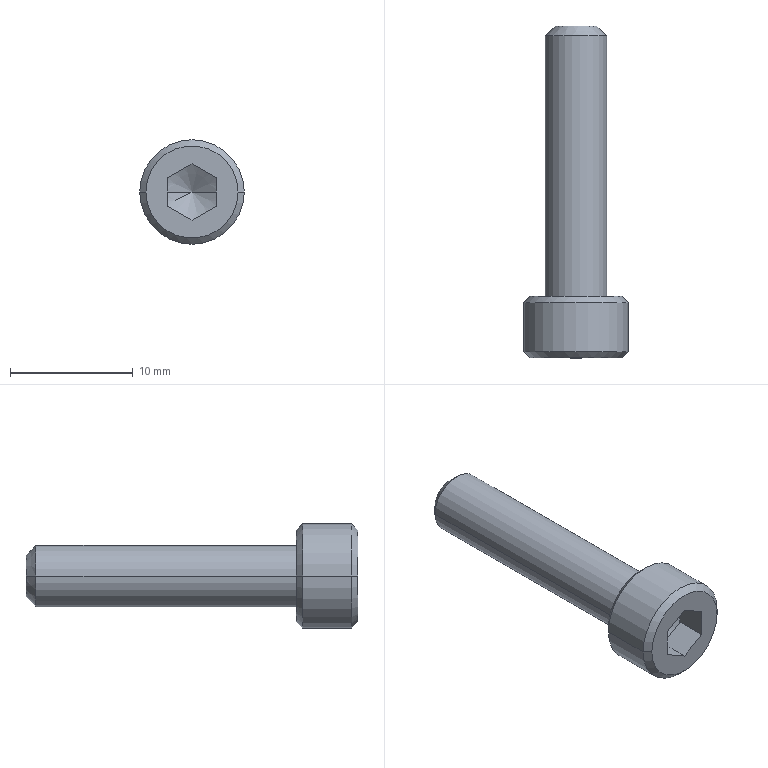Part | STEP file | BB62-M5-22L-44 | 1 solid | 27 faces | box 8.5 x 27 x 8.5 mm | volume 663.468 mm3 | plane 15 | cone 8 | cylinder 4 | commonest cylinder face diameters 5 x2 8.5 x2
STEP:
#1=CARTESIAN_POINT('',(0.,-1.178,0.));
#2=VERTEX_POINT('',#1);
#3=CARTESIAN_POINT('',(2.29,-2.5,0.));
#4=VERTEX_POINT('',#3);
#5=CARTESIAN_POINT('',(0.,-1.178,0.));
#6=DIRECTION('',(0.866,-0.5,0.));
#7=VECTOR('',#6,1000.);
#8=LINE('',#5,#7);
#9=EDGE_CURVE('',#2,#4,#8,.T.);
#10=ORIENTED_EDGE('',*,*,#9,.F.);
#11=CARTESIAN_POINT('',(-2.29,-2.5,0.));
#12=VERTEX_POINT('',#11);
#13=CARTESIAN_POINT('',(0.,-1.178,0.));
#14=DIRECTION('',(-0.866,-0.5,0.));
#15=VECTOR('',#14,1000.);
#16=LINE('',#13,#15);
#17=EDGE_CURVE('',#2,#12,#16,.T.);
#18=ORIENTED_EDGE('',*,*,#17,.T.);
#19=CARTESIAN_POINT('',(-1.983,-2.5,-1.145));
#20=VERTEX_POINT('',#19);
#21=CARTESIAN_POINT('',(0.,-2.5,0.));
#22=DIRECTION('',(0.,-1.,0.));
#23=DIRECTION('',(-1.,0.,0.));
#24=AXIS2_PLACEMENT_3D('',#21,#22,#23);
#25=CIRCLE('',#24,2.29);
#26=EDGE_CURVE('',#12,#20,#25,.T.);
#27=ORIENTED_EDGE('',*,*,#26,.T.);
#28=CARTESIAN_POINT('',(0.,-2.5,-2.29));
#29=VERTEX_POINT('',#28);
#30=CARTESIAN_POINT('',(0.,-2.5,0.));
#31=DIRECTION('',(0.,-1.,0.));
#32=DIRECTION('',(-1.,0.,0.));
#33=AXIS2_PLACEMENT_3D('',#30,#31,#32);
#34=CIRCLE('',#33,2.29);
#35=EDGE_CURVE('',#20,#29,#34,.T.);
#36=ORIENTED_EDGE('',*,*,#35,.T.);
#37=CARTESIAN_POINT('',(1.983,-2.5,-1.145));
#38=VERTEX_POINT('',#37);
#39=CARTESIAN_POINT('',(0.,-2.5,0.));
#40=DIRECTION('',(0.,-1.,0.));
#41=DIRECTION('',(-1.,0.,0.));
#42=AXIS2_PLACEMENT_3D('',#39,#40,#41);
#43=CIRCLE('',#42,2.29);
#44=EDGE_CURVE('',#29,#38,#43,.T.);
#45=ORIENTED_EDGE('',*,*,#44,.T.);
#46=CARTESIAN_POINT('',(0.,-2.5,0.));
#47=DIRECTION('',(0.,-1.,0.));
#48=DIRECTION('',(-1.,0.,0.));
#49=AXIS2_PLACEMENT_3D('',#46,#47,#48);
#50=CIRCLE('',#49,2.29);
#51=EDGE_CURVE('',#38,#4,#50,.T.);
#52=ORIENTED_EDGE('',*,*,#51,.T.);
#53=EDGE_LOOP('',(#10,#18,#27,#36,#45,#52));
#54=FACE_OUTER_BOUND('',#53,.T.);
#55=CARTESIAN_POINT('',(0.,-1001.178,0.));
#56=DIRECTION('',(0.,-1.,0.));
#57=DIRECTION('',(1.,0.,0.));
#58=AXIS2_PLACEMENT_3D('',#55,#56,#57);
#59=CONICAL_SURFACE('',#58,1732.051,1.047);
#60=ADVANCED_FACE('',(#54),#59,.F.);
#61=CARTESIAN_POINT('',(-1.7,22.,0.));
#62=VERTEX_POINT('',#61);
#63=CARTESIAN_POINT('',(1.7,22.,0.));
#64=VERTEX_POINT('',#63);
#65=CARTESIAN_POINT('',(0.,22.,0.));
#66=DIRECTION('',(0.,1.,0.));
#67=DIRECTION('',(1.,0.,0.));
#68=AXIS2_PLACEMENT_3D('',#65,#66,#67);
#69=CIRCLE('',#68,1.7);
#70=EDGE_CURVE('',#62,#64,#69,.T.);
#71=ORIENTED_EDGE('',*,*,#70,.F.);
#72=CARTESIAN_POINT('',(-2.5,21.2,0.));
#73=VERTEX_POINT('',#72);
#74=CARTESIAN_POINT('',(-1.7,22.,0.));
#75=DIRECTION('',(-0.7071,-0.7071,0.));
#76=VECTOR('',#75,1000.);
#77=LINE('',#74,#76);
#78=EDGE_CURVE('',#62,#73,#77,.T.);
#79=ORIENTED_EDGE('',*,*,#78,.T.);
#80=CARTESIAN_POINT('',(2.5,21.2,0.));
#81=VERTEX_POINT('',#80);
#82=CARTESIAN_POINT('',(0.,21.2,0.));
#83=DIRECTION('',(0.,-1.,0.));
#84=DIRECTION('',(-1.,0.,0.));
#85=AXIS2_PLACEMENT_3D('',#82,#83,#84);
#86=CIRCLE('',#85,2.5);
#87=EDGE_CURVE('',#81,#73,#86,.T.);
#88=ORIENTED_EDGE('',*,*,#87,.F.);
#89=CARTESIAN_POINT('',(1.7,22.,0.));
#90=DIRECTION('',(0.7071,-0.7071,0.));
#91=VECTOR('',#90,1000.);
#92=LINE('',#89,#91);
#93=EDGE_CURVE('',#64,#81,#92,.T.);
#94=ORIENTED_EDGE('',*,*,#93,.F.);
#95=EDGE_LOOP('',(#71,#79,#88,#94));
#96=FACE_OUTER_BOUND('',#95,.T.);
#97=CARTESIAN_POINT('',(0.,22.,0.));
#98=DIRECTION('',(0.,-1.,0.));
#99=DIRECTION('',(1.,0.,0.));
#100=AXIS2_PLACEMENT_3D('',#97,#98,#99);
#101=CONICAL_SURFACE('',#100,1.7,0.7854);
#102=ADVANCED_FACE('',(#96),#101,.T.);
#103=ORIENTED_EDGE('',*,*,#87,.T.);
#104=CARTESIAN_POINT('',(-2.5,0.,0.));
#105=VERTEX_POINT('',#104);
#106=CARTESIAN_POINT('',(-2.5,21.2,0.));
#107=DIRECTION('',(0.,-1.,0.));
#108=VECTOR('',#107,1000.);
#109=LINE('',#106,#108);
#110=EDGE_CURVE('',#73,#105,#109,.T.);
#111=ORIENTED_EDGE('',*,*,#110,.T.);
#112=CARTESIAN_POINT('',(2.5,0.,0.));
#113=VERTEX_POINT('',#112);
#114=CARTESIAN_POINT('',(0.,0.,0.));
#115=DIRECTION('',(0.,-1.,0.));
#116=DIRECTION('',(-1.,0.,0.));
#117=AXIS2_PLACEMENT_3D('',#114,#115,#116);
#118=CIRCLE('',#117,2.5);
#119=EDGE_CURVE('',#113,#105,#118,.T.);
#120=ORIENTED_EDGE('',*,*,#119,.F.);
#121=CARTESIAN_POINT('',(2.5,21.2,0.));
#122=DIRECTION('',(0.,-1.,0.));
#123=VECTOR('',#122,1000.);
#124=LINE('',#121,#123);
#125=EDGE_CURVE('',#81,#113,#124,.T.);
#126=ORIENTED_EDGE('',*,*,#125,.F.);
#127=EDGE_LOOP('',(#103,#111,#120,#126));
#128=FACE_OUTER_BOUND('',#127,.T.);
#129=CARTESIAN_POINT('',(0.,21.2,0.));
#130=DIRECTION('',(0.,-1.,0.));
#131=DIRECTION('',(1.,0.,0.));
#132=AXIS2_PLACEMENT_3D('',#129,#130,#131);
#133=CYLINDRICAL_SURFACE('',#132,2.5);
#134=ADVANCED_FACE('',(#128),#133,.T.);
#135=CARTESIAN_POINT('',(3.75,-5.,0.));
#136=VERTEX_POINT('',#135);
#137=CARTESIAN_POINT('',(-3.75,-5.,0.));
#138=VERTEX_POINT('',#137);
#139=CARTESIAN_POINT('',(0.,-5.,0.));
#140=DIRECTION('',(0.,-1.,0.));
#141=DIRECTION('',(-1.,0.,0.));
#142=AXIS2_PLACEMENT_3D('',#139,#140,#141);
#143=CIRCLE('',#142,3.75);
#144=EDGE_CURVE('',#136,#138,#143,.T.);
#145=ORIENTED_EDGE('',*,*,#144,.F.);
#146=CARTESIAN_POINT('',(4.25,-4.5,0.));
#147=VERTEX_POINT('',#146);
#148=CARTESIAN_POINT('',(4.25,-4.5,0.));
#149=DIRECTION('',(0.7071,0.7071,0.));
#150=VECTOR('',#149,1000.);
#151=LINE('',#148,#150);
#152=EDGE_CURVE('',#136,#147,#151,.T.);
#153=ORIENTED_EDGE('',*,*,#152,.T.);
#154=CARTESIAN_POINT('',(-4.25,-4.5,0.));
#155=VERTEX_POINT('',#154);
#156=CARTESIAN_POINT('',(0.,-4.5,0.));
#157=DIRECTION('',(0.,-1.,0.));
#158=DIRECTION('',(-1.,0.,0.));
#159=AXIS2_PLACEMENT_3D('',#156,#157,#158);
#160=CIRCLE('',#159,4.25);
#161=EDGE_CURVE('',#147,#155,#160,.T.);
#162=ORIENTED_EDGE('',*,*,#161,.T.);
#163=CARTESIAN_POINT('',(-4.25,-4.5,0.));
#164=DIRECTION('',(-0.7071,0.7071,0.));
#165=VECTOR('',#164,1000.);
#166=LINE('',#163,#165);
#167=EDGE_CURVE('',#138,#155,#166,.T.);
#168=ORIENTED_EDGE('',*,*,#167,.F.);
#169=EDGE_LOOP('',(#145,#153,#162,#168));
#170=FACE_OUTER_BOUND('',#169,.T.);
#171=CARTESIAN_POINT('',(0.,-4.5,0.));
#172=DIRECTION('',(0.,1.,0.));
#173=DIRECTION('',(-1.,0.,0.));
#174=AXIS2_PLACEMENT_3D('',#171,#172,#173);
#175=CONICAL_SURFACE('',#174,4.25,0.7854);
#176=ADVANCED_FACE('',(#170),#175,.T.);
#177=ORIENTED_EDGE('',*,*,#161,.F.);
#178=CARTESIAN_POINT('',(4.25,-0.5,0.));
#179=VERTEX_POINT('',#178);
#180=CARTESIAN_POINT('',(4.25,-1.62,0.));
#181=DIRECTION('',(0.,1.,0.));
#182=VECTOR('',#181,1000.);
#183=LINE('',#180,#182);
#184=EDGE_CURVE('',#147,#179,#183,.T.);
#185=ORIENTED_EDGE('',*,*,#184,.T.);
#186=CARTESIAN_POINT('',(-4.25,-0.5,0.));
#187=VERTEX_POINT('',#186);
#188=CARTESIAN_POINT('',(0.,-0.5,0.));
#189=DIRECTION('',(0.,-1.,0.));
#190=DIRECTION('',(-1.,0.,0.));
#191=AXIS2_PLACEMENT_3D('',#188,#189,#190);
#192=CIRCLE('',#191,4.25);
#193=EDGE_CURVE('',#179,#187,#192,.T.);
#194=ORIENTED_EDGE('',*,*,#193,.T.);
#195=CARTESIAN_POINT('',(-4.25,-1.62,0.));
#196=DIRECTION('',(0.,1.,0.));
#197=VECTOR('',#196,1000.);
#198=LINE('',#195,#197);
#199=EDGE_CURVE('',#155,#187,#198,.T.);
#200=ORIENTED_EDGE('',*,*,#199,.F.);
#201=EDGE_LOOP('',(#177,#185,#194,#200));
#202=FACE_OUTER_BOUND('',#201,.T.);
#203=CARTESIAN_POINT('',(0.,-1.62,0.));
#204=DIRECTION('',(0.,1.,0.));
#205=DIRECTION('',(-1.,0.,0.));
#206=AXIS2_PLACEMENT_3D('',#203,#204,#205);
#207=CYLINDRICAL_SURFACE('',#206,4.25);
#208=ADVANCED_FACE('',(#202),#207,.T.);
#209=CARTESIAN_POINT('',(3.75,0.,0.));
#210=VERTEX_POINT('',#209);
#211=CARTESIAN_POINT('',(-3.75,0.,0.));
#212=VERTEX_POINT('',#211);
#213=CARTESIAN_POINT('',(0.,0.,0.));
#214=DIRECTION('',(0.,-1.,0.));
#215=DIRECTION('',(-1.,0.,0.));
#216=AXIS2_PLACEMENT_3D('',#213,#214,#215);
#217=CIRCLE('',#216,3.75);
#218=EDGE_CURVE('',#210,#212,#217,.T.);
#219=ORIENTED_EDGE('',*,*,#218,.T.);
#220=CARTESIAN_POINT('',(-3.75,0.,0.));
#221=DIRECTION('',(-0.7071,-0.7071,0.));
#222=VECTOR('',#221,1000.);
#223=LINE('',#220,#222);
#224=EDGE_CURVE('',#212,#187,#223,.T.);
#225=ORIENTED_EDGE('',*,*,#224,.T.);
#226=ORIENTED_EDGE('',*,*,#193,.F.);
#227=CARTESIAN_POINT('',(3.75,0.,0.));
#228=DIRECTION('',(0.7071,-0.7071,0.));
#229=VECTOR('',#228,1000.);
#230=LINE('',#227,#229);
#231=EDGE_CURVE('',#210,#179,#230,.T.);
#232=ORIENTED_EDGE('',*,*,#231,.F.);
#233=EDGE_LOOP('',(#219,#225,#226,#232));
#234=FACE_OUTER_BOUND('',#233,.T.);
#235=CARTESIAN_POINT('',(0.,0.,0.));
#236=DIRECTION('',(0.,-1.,0.));
#237=DIRECTION('',(1.,0.,0.));
#238=AXIS2_PLACEMENT_3D('',#235,#236,#237);
#239=CONICAL_SURFACE('',#238,3.75,0.7854);
#240=ADVANCED_FACE('',(#234),#239,.T.);
#241=CARTESIAN_POINT('',(0.,-5.,0.));
#242=DIRECTION('',(0.,-1.,0.));
#243=DIRECTION('',(-1.,0.,0.));
#244=AXIS2_PLACEMENT_3D('',#241,#242,#243);
#245=CIRCLE('',#244,3.75);
#246=EDGE_CURVE('',#138,#136,#245,.T.);
#247=ORIENTED_EDGE('',*,*,#246,.T.);
#248=ORIENTED_EDGE('',*,*,#144,.T.);
#249=EDGE_LOOP('',(#247,#248));
#250=FACE_OUTER_BOUND('',#249,.T.);
#251=CARTESIAN_POINT('',(0.,-5.,-2.29));
#252=VERTEX_POINT('',#251);
#253=CARTESIAN_POINT('',(-1.983,-5.,-1.145));
#254=VERTEX_POINT('',#253);
#255=CARTESIAN_POINT('',(0.,-5.,-2.29));
#256=DIRECTION('',(-0.866,0.,0.5));
#257=VECTOR('',#256,1000.);
#258=LINE('',#255,#257);
#259=EDGE_CURVE('',#252,#254,#258,.T.);
#260=ORIENTED_EDGE('',*,*,#259,.T.);
#261=CARTESIAN_POINT('',(-1.983,-5.,1.145));
#262=VERTEX_POINT('',#261);
#263=CARTESIAN_POINT('',(-1.983,-5.,-1.145));
#264=DIRECTION('',(0.,0.,1.));
#265=VECTOR('',#264,1000.);
#266=LINE('',#263,#265);
#267=EDGE_CURVE('',#254,#262,#266,.T.);
#268=ORIENTED_EDGE('',*,*,#267,.T.);
#269=CARTESIAN_POINT('',(0.,-5.,2.29));
#270=VERTEX_POINT('',#269);
#271=CARTESIAN_POINT('',(-1.983,-5.,1.145));
#272=DIRECTION('',(0.866,0.,0.5));
#273=VECTOR('',#272,1000.);
#274=LINE('',#271,#273);
#275=EDGE_CURVE('',#262,#270,#274,.T.);
#276=ORIENTED_EDGE('',*,*,#275,.T.);
#277=CARTESIAN_POINT('',(1.983,-5.,1.145));
#278=VERTEX_POINT('',#277);
#279=CARTESIAN_POINT('',(0.,-5.,2.29));
#280=DIRECTION('',(0.866,0.,-0.5));
#281=VECTOR('',#280,1000.);
#282=LINE('',#279,#281);
#283=EDGE_CURVE('',#270,#278,#282,.T.);
#284=ORIENTED_EDGE('',*,*,#283,.T.);
#285=CARTESIAN_POINT('',(1.983,-5.,-1.145));
#286=VERTEX_POINT('',#285);
#287=CARTESIAN_POINT('',(1.983,-5.,1.145));
#288=DIRECTION('',(0.,0.,-1.));
#289=VECTOR('',#288,1000.);
#290=LINE('',#287,#289);
#291=EDGE_CURVE('',#278,#286,#290,.T.);
#292=ORIENTED_EDGE('',*,*,#291,.T.);
#293=CARTESIAN_POINT('',(1.983,-5.,-1.145));
#294=DIRECTION('',(-0.866,0.,-0.5));
#295=VECTOR('',#294,1000.);
#296=LINE('',#293,#295);
#297=EDGE_CURVE('',#286,#252,#296,.T.);
#298=ORIENTED_EDGE('',*,*,#297,.T.);
#299=EDGE_LOOP('',(#260,#268,#276,#284,#292,#298));
#300=FACE_BOUND('',#299,.T.);
#301=CARTESIAN_POINT('',(3.75,-5.,0.));
#302=DIRECTION('',(0.,-1.,0.));
#303=DIRECTION('',(1.,0.,0.));
#304=AXIS2_PLACEMENT_3D('',#301,#302,#303);
#305=PLANE('',#304);
#306=ADVANCED_FACE('',(#250,#300),#305,.T.);
#307=ORIENTED_EDGE('',*,*,#119,.T.);
#308=CARTESIAN_POINT('',(0.,0.,0.));
#309=DIRECTION('',(0.,-1.,0.));
#310=DIRECTION('',(-1.,0.,0.));
#311=AXIS2_PLACEMENT_3D('',#308,#309,#310);
#312=CIRCLE('',#311,2.5);
#313=EDGE_CURVE('',#105,#113,#312,.T.);
#314=ORIENTED_EDGE('',*,*,#313,.T.);
#315=EDGE_LOOP('',(#307,#314));
#316=FACE_BOUND('',#315,.T.);
#317=ORIENTED_EDGE('',*,*,#218,.F.);
#318=CARTESIAN_POINT('',(0.,0.,0.));
#319=DIRECTION('',(0.,-1.,0.));
#320=DIRECTION('',(-1.,0.,0.));
#321=AXIS2_PLACEMENT_3D('',#318,#319,#320);
#322=CIRCLE('',#321,3.75);
#323=EDGE_CURVE('',#212,#210,#322,.T.);
#324=ORIENTED_EDGE('',*,*,#323,.F.);
#325=EDGE_LOOP('',(#317,#324));
#326=FACE_OUTER_BOUND('',#325,.T.);
#327=CARTESIAN_POINT('',(0.,0.,0.));
#328=DIRECTION('',(0.,1.,0.));
#329=DIRECTION('',(-1.,0.,0.));
#330=AXIS2_PLACEMENT_3D('',#327,#328,#329);
#331=PLANE('',#330);
#332=ADVANCED_FACE('',(#316,#326),#331,.T.);
#333=ORIENTED_EDGE('',*,*,#224,.F.);
#334=ORIENTED_EDGE('',*,*,#323,.T.);
#335=ORIENTED_EDGE('',*,*,#231,.T.);
#336=CARTESIAN_POINT('',(0.,-0.5,0.));
#337=DIRECTION('',(0.,-1.,0.));
#338=DIRECTION('',(-1.,0.,0.));
#339=AXIS2_PLACEMENT_3D('',#336,#337,#338);
#340=CIRCLE('',#339,4.25);
#341=EDGE_CURVE('',#187,#179,#340,.T.);
#342=ORIENTED_EDGE('',*,*,#341,.F.);
#343=EDGE_LOOP('',(#333,#334,#335,#342));
#344=FACE_OUTER_BOUND('',#343,.T.);
#345=CARTESIAN_POINT('',(0.,0.,0.));
#346=DIRECTION('',(0.,-1.,0.));
#347=DIRECTION('',(1.,0.,0.));
#348=AXIS2_PLACEMENT_3D('',#345,#346,#347);
#349=CONICAL_SURFACE('',#348,3.75,0.7854);
#350=ADVANCED_FACE('',(#344),#349,.T.);
#351=ORIENTED_EDGE('',*,*,#184,.F.);
#352=CARTESIAN_POINT('',(0.,-4.5,0.));
#353=DIRECTION('',(0.,-1.,0.));
#354=DIRECTION('',(-1.,0.,0.));
#355=AXIS2_PLACEMENT_3D('',#352,#353,#354);
#356=CIRCLE('',#355,4.25);
#357=EDGE_CURVE('',#155,#147,#356,.T.);
#358=ORIENTED_EDGE('',*,*,#357,.F.);
#359=ORIENTED_EDGE('',*,*,#199,.T.);
#360=ORIENTED_EDGE('',*,*,#341,.T.);
#361=EDGE_LOOP('',(#351,#358,#359,#360));
#362=FACE_OUTER_BOUND('',#361,.T.);
#363=CARTESIAN_POINT('',(0.,-1.62,0.));
#364=DIRECTION('',(0.,1.,0.));
#365=DIRECTION('',(-1.,0.,0.));
#366=AXIS2_PLACEMENT_3D('',#363,#364,#365);
#367=CYLINDRICAL_SURFACE('',#366,4.25);
#368=ADVANCED_FACE('',(#362),#367,.T.);
#369=ORIENTED_EDGE('',*,*,#152,.F.);
#370=ORIENTED_EDGE('',*,*,#246,.F.);
#371=ORIENTED_EDGE('',*,*,#167,.T.);
#372=ORIENTED_EDGE('',*,*,#357,.T.);
#373=EDGE_LOOP('',(#369,#370,#371,#372));
#374=FACE_OUTER_BOUND('',#373,.T.);
#375=CARTESIAN_POINT('',(0.,-4.5,0.));
#376=DIRECTION('',(0.,1.,0.));
#377=DIRECTION('',(-1.,0.,0.));
#378=AXIS2_PLACEMENT_3D('',#375,#376,#377);
#379=CONICAL_SURFACE('',#378,4.25,0.7854);
#380=ADVANCED_FACE('',(#374),#379,.T.);
#381=ORIENTED_EDGE('',*,*,#110,.F.);
#382=CARTESIAN_POINT('',(0.,21.2,0.));
#383=DIRECTION('',(0.,-1.,0.));
#384=DIRECTION('',(-1.,0.,0.));
#385=AXIS2_PLACEMENT_3D('',#382,#383,#384);
#386=CIRCLE('',#385,2.5);
#387=EDGE_CURVE('',#73,#81,#386,.T.);
#388=ORIENTED_EDGE('',*,*,#387,.T.);
#389=ORIENTED_EDGE('',*,*,#125,.T.);
#390=ORIENTED_EDGE('',*,*,#313,.F.);
#391=EDGE_LOOP('',(#381,#388,#389,#390));
#392=FACE_OUTER_BOUND('',#391,.T.);
#393=CARTESIAN_POINT('',(0.,21.2,0.));
#394=DIRECTION('',(0.,-1.,0.));
#395=DIRECTION('',(1.,0.,0.));
#396=AXIS2_PLACEMENT_3D('',#393,#394,#395);
#397=CYLINDRICAL_SURFACE('',#396,2.5);
#398=ADVANCED_FACE('',(#392),#397,.T.);
#399=CARTESIAN_POINT('',(0.,22.,0.));
#400=DIRECTION('',(0.,1.,0.));
#401=DIRECTION('',(1.,0.,0.));
#402=AXIS2_PLACEMENT_3D('',#399,#400,#401);
#403=CIRCLE('',#402,1.7);
#404=EDGE_CURVE('',#64,#62,#403,.T.);
#405=ORIENTED_EDGE('',*,*,#404,.T.);
#406=ORIENTED_EDGE('',*,*,#70,.T.);
#407=EDGE_LOOP('',(#405,#406));
#408=FACE_OUTER_BOUND('',#407,.T.);
#409=CARTESIAN_POINT('',(0.,22.,0.));
#410=DIRECTION('',(0.,1.,0.));
#411=DIRECTION('',(-1.,0.,0.));
#412=AXIS2_PLACEMENT_3D('',#409,#410,#411);
#413=PLANE('',#412);
#414=ADVANCED_FACE('',(#408),#413,.T.);
#415=ORIENTED_EDGE('',*,*,#78,.F.);
#416=ORIENTED_EDGE('',*,*,#404,.F.);
#417=ORIENTED_EDGE('',*,*,#93,.T.);
#418=ORIENTED_EDGE('',*,*,#387,.F.);
#419=EDGE_LOOP('',(#415,#416,#417,#418));
#420=FACE_OUTER_BOUND('',#419,.T.);
#421=CARTESIAN_POINT('',(0.,22.,0.));
#422=DIRECTION('',(0.,-1.,0.));
#423=DIRECTION('',(1.,0.,0.));
#424=AXIS2_PLACEMENT_3D('',#421,#422,#423);
#425=CONICAL_SURFACE('',#424,1.7,0.7854);
#426=ADVANCED_FACE('',(#420),#425,.T.);
#427=CARTESIAN_POINT('',(1.983,-2.5,-1.145));
#428=DIRECTION('',(-0.866,0.,-0.5));
#429=VECTOR('',#428,1000.);
#430=LINE('',#427,#429);
#431=EDGE_CURVE('',#38,#29,#430,.T.);
#432=ORIENTED_EDGE('',*,*,#431,.T.);
#433=CARTESIAN_POINT('',(0.,-5.,-2.29));
#434=DIRECTION('',(0.,1.,0.));
#435=VECTOR('',#434,1000.);
#436=LINE('',#433,#435);
#437=EDGE_CURVE('',#252,#29,#436,.T.);
#438=ORIENTED_EDGE('',*,*,#437,.F.);
#439=ORIENTED_EDGE('',*,*,#297,.F.);
#440=CARTESIAN_POINT('',(1.983,-5.,-1.145));
#441=DIRECTION('',(0.,1.,0.));
#442=VECTOR('',#441,1000.);
#443=LINE('',#440,#442);
#444=EDGE_CURVE('',#286,#38,#443,.T.);
#445=ORIENTED_EDGE('',*,*,#444,.T.);
#446=EDGE_LOOP('',(#432,#438,#439,#445));
#447=FACE_OUTER_BOUND('',#446,.T.);
#448=CARTESIAN_POINT('',(1.983,-5.,-1.145));
#449=DIRECTION('',(-0.5,0.,0.866));
#450=DIRECTION('',(0.866,0.,0.5));
#451=AXIS2_PLACEMENT_3D('',#448,#449,#450);
#452=PLANE('',#451);
#453=ADVANCED_FACE('',(#447),#452,.T.);
#454=CARTESIAN_POINT('',(0.,-2.5,-2.29));
#455=DIRECTION('',(-0.866,0.,0.5));
#456=VECTOR('',#455,1000.);
#457=LINE('',#454,#456);
#458=EDGE_CURVE('',#29,#20,#457,.T.);
#459=ORIENTED_EDGE('',*,*,#458,.T.);
#460=CARTESIAN_POINT('',(-1.983,-5.,-1.145));
#461=DIRECTION('',(0.,1.,0.));
#462=VECTOR('',#461,1000.);
#463=LINE('',#460,#462);
#464=EDGE_CURVE('',#254,#20,#463,.T.);
#465=ORIENTED_EDGE('',*,*,#464,.F.);
#466=ORIENTED_EDGE('',*,*,#259,.F.);
#467=ORIENTED_EDGE('',*,*,#437,.T.);
#468=EDGE_LOOP('',(#459,#465,#466,#467));
#469=FACE_OUTER_BOUND('',#468,.T.);
#470=CARTESIAN_POINT('',(0.,-5.,-2.29));
#471=DIRECTION('',(0.5,0.,0.866));
#472=DIRECTION('',(0.866,0.,-0.5));
#473=AXIS2_PLACEMENT_3D('',#470,#471,#472);
#474=PLANE('',#473);
#475=ADVANCED_FACE('',(#469),#474,.T.);
#476=CARTESIAN_POINT('',(-1.983,-2.5,1.145));
#477=VERTEX_POINT('',#476);
#478=CARTESIAN_POINT('',(-1.983,-2.5,-1.145));
#479=DIRECTION('',(0.,0.,1.));
#480=VECTOR('',#479,1000.);
#481=LINE('',#478,#480);
#482=EDGE_CURVE('',#20,#477,#481,.T.);
#483=ORIENTED_EDGE('',*,*,#482,.T.);
#484=CARTESIAN_POINT('',(-1.983,-5.,1.145));
#485=DIRECTION('',(0.,1.,0.));
#486=VECTOR('',#485,1000.);
#487=LINE('',#484,#486);
#488=EDGE_CURVE('',#262,#477,#487,.T.);
#489=ORIENTED_EDGE('',*,*,#488,.F.);
#490=ORIENTED_EDGE('',*,*,#267,.F.);
#491=ORIENTED_EDGE('',*,*,#464,.T.);
#492=EDGE_LOOP('',(#483,#489,#490,#491));
#493=FACE_OUTER_BOUND('',#492,.T.);
#494=CARTESIAN_POINT('',(-1.983,-5.,-1.145));
#495=DIRECTION('',(1.,0.,0.));
#496=DIRECTION('',(0.,0.,-1.));
#497=AXIS2_PLACEMENT_3D('',#494,#495,#496);
#498=PLANE('',#497);
#499=ADVANCED_FACE('',(#493),#498,.T.);
#500=CARTESIAN_POINT('',(0.,-2.5,2.29));
#501=VERTEX_POINT('',#500);
#502=CARTESIAN_POINT('',(-1.983,-2.5,1.145));
#503=DIRECTION('',(0.866,0.,0.5));
#504=VECTOR('',#503,1000.);
#505=LINE('',#502,#504);
#506=EDGE_CURVE('',#477,#501,#505,.T.);
#507=ORIENTED_EDGE('',*,*,#506,.T.);
#508=CARTESIAN_POINT('',(0.,-5.,2.29));
#509=DIRECTION('',(0.,1.,0.));
#510=VECTOR('',#509,1000.);
#511=LINE('',#508,#510);
#512=EDGE_CURVE('',#270,#501,#511,.T.);
#513=ORIENTED_EDGE('',*,*,#512,.F.);
#514=ORIENTED_EDGE('',*,*,#275,.F.);
#515=ORIENTED_EDGE('',*,*,#488,.T.);
#516=EDGE_LOOP('',(#507,#513,#514,#515));
#517=FACE_OUTER_BOUND('',#516,.T.);
#518=CARTESIAN_POINT('',(-1.983,-5.,1.145));
#519=DIRECTION('',(0.5,0.,-0.866));
#520=DIRECTION('',(-0.866,0.,-0.5));
#521=AXIS2_PLACEMENT_3D('',#518,#519,#520);
#522=PLANE('',#521);
#523=ADVANCED_FACE('',(#517),#522,.T.);
#524=CARTESIAN_POINT('',(1.983,-2.5,1.145));
#525=VERTEX_POINT('',#524);
#526=CARTESIAN_POINT('',(0.,-2.5,2.29));
#527=DIRECTION('',(0.866,0.,-0.5));
#528=VECTOR('',#527,1000.);
#529=LINE('',#526,#528);
#530=EDGE_CURVE('',#501,#525,#529,.T.);
#531=ORIENTED_EDGE('',*,*,#530,.T.);
#532=CARTESIAN_POINT('',(1.983,-5.,1.145));
#533=DIRECTION('',(0.,1.,0.));
#534=VECTOR('',#533,1000.);
#535=LINE('',#532,#534);
#536=EDGE_CURVE('',#278,#525,#535,.T.);
#537=ORIENTED_EDGE('',*,*,#536,.F.);
#538=ORIENTED_EDGE('',*,*,#283,.F.);
#539=ORIENTED_EDGE('',*,*,#512,.T.);
#540=EDGE_LOOP('',(#531,#537,#538,#539));
#541=FACE_OUTER_BOUND('',#540,.T.);
#542=CARTESIAN_POINT('',(0.,-5.,2.29));
#543=DIRECTION('',(-0.5,0.,-0.866));
#544=DIRECTION('',(-0.866,0.,0.5));
#545=AXIS2_PLACEMENT_3D('',#542,#543,#544);
#546=PLANE('',#545);
#547=ADVANCED_FACE('',(#541),#546,.T.);
#548=CARTESIAN_POINT('',(1.983,-2.5,1.145));
#549=DIRECTION('',(0.,0.,-1.));
#550=VECTOR('',#549,1000.);
#551=LINE('',#548,#550);
#552=EDGE_CURVE('',#525,#38,#551,.T.);
#553=ORIENTED_EDGE('',*,*,#552,.T.);
#554=ORIENTED_EDGE('',*,*,#444,.F.);
#555=ORIENTED_EDGE('',*,*,#291,.F.);
#556=ORIENTED_EDGE('',*,*,#536,.T.);
#557=EDGE_LOOP('',(#553,#554,#555,#556));
#558=FACE_OUTER_BOUND('',#557,.T.);
#559=CARTESIAN_POINT('',(1.983,-5.,1.145));
#560=DIRECTION('',(-1.,0.,0.));
#561=DIRECTION('',(0.,0.,1.));
#562=AXIS2_PLACEMENT_3D('',#559,#560,#561);
#563=PLANE('',#562);
#564=ADVANCED_FACE('',(#558),#563,.T.);
#565=ORIENTED_EDGE('',*,*,#431,.F.);
#566=ORIENTED_EDGE('',*,*,#44,.F.);
#567=EDGE_LOOP('',(#565,#566));
#568=FACE_OUTER_BOUND('',#567,.T.);
#569=CARTESIAN_POINT('',(0.,-2.5,0.));
#570=DIRECTION('',(0.,-1.,0.));
#571=DIRECTION('',(1.,0.,0.));
#572=AXIS2_PLACEMENT_3D('',#569,#570,#571);
#573=PLANE('',#572);
#574=ADVANCED_FACE('',(#568),#573,.F.);
#575=ORIENTED_EDGE('',*,*,#552,.F.);
#576=CARTESIAN_POINT('',(0.,-2.5,0.));
#577=DIRECTION('',(0.,-1.,0.));
#578=DIRECTION('',(-1.,0.,0.));
#579=AXIS2_PLACEMENT_3D('',#576,#577,#578);
#580=CIRCLE('',#579,2.29);
#581=EDGE_CURVE('',#4,#525,#580,.T.);
#582=ORIENTED_EDGE('',*,*,#581,.F.);
#583=ORIENTED_EDGE('',*,*,#51,.F.);
#584=EDGE_LOOP('',(#575,#582,#583));
#585=FACE_OUTER_BOUND('',#584,.T.);
#586=CARTESIAN_POINT('',(0.,-2.5,0.));
#587=DIRECTION('',(0.,-1.,0.));
#588=DIRECTION('',(1.,0.,0.));
#589=AXIS2_PLACEMENT_3D('',#586,#587,#588);
#590=PLANE('',#589);
#591=ADVANCED_FACE('',(#585),#590,.F.);
#592=ORIENTED_EDGE('',*,*,#530,.F.);
#593=CARTESIAN_POINT('',(0.,-2.5,0.));
#594=DIRECTION('',(0.,-1.,0.));
#595=DIRECTION('',(-1.,0.,0.));
#596=AXIS2_PLACEMENT_3D('',#593,#594,#595);
#597=CIRCLE('',#596,2.29);
#598=EDGE_CURVE('',#525,#501,#597,.T.);
#599=ORIENTED_EDGE('',*,*,#598,.F.);
#600=EDGE_LOOP('',(#592,#599));
#601=FACE_OUTER_BOUND('',#600,.T.);
#602=CARTESIAN_POINT('',(0.,-2.5,0.));
#603=DIRECTION('',(0.,-1.,0.));
#604=DIRECTION('',(1.,0.,0.));
#605=AXIS2_PLACEMENT_3D('',#602,#603,#604);
#606=PLANE('',#605);
#607=ADVANCED_FACE('',(#601),#606,.F.);
#608=ORIENTED_EDGE('',*,*,#506,.F.);
#609=CARTESIAN_POINT('',(0.,-2.5,0.));
#610=DIRECTION('',(0.,-1.,0.));
#611=DIRECTION('',(-1.,0.,0.));
#612=AXIS2_PLACEMENT_3D('',#609,#610,#611);
#613=CIRCLE('',#612,2.29);
#614=EDGE_CURVE('',#501,#477,#613,.T.);
#615=ORIENTED_EDGE('',*,*,#614,.F.);
#616=EDGE_LOOP('',(#608,#615));
#617=FACE_OUTER_BOUND('',#616,.T.);
#618=CARTESIAN_POINT('',(0.,-2.5,0.));
#619=DIRECTION('',(0.,-1.,0.));
#620=DIRECTION('',(1.,0.,0.));
#621=AXIS2_PLACEMENT_3D('',#618,#619,#620);
#622=PLANE('',#621);
#623=ADVANCED_FACE('',(#617),#622,.F.);
#624=ORIENTED_EDGE('',*,*,#482,.F.);
#625=ORIENTED_EDGE('',*,*,#26,.F.);
#626=CARTESIAN_POINT('',(0.,-2.5,0.));
#627=DIRECTION('',(0.,-1.,0.));
#628=DIRECTION('',(-1.,0.,0.));
#629=AXIS2_PLACEMENT_3D('',#626,#627,#628);
#630=CIRCLE('',#629,2.29);
#631=EDGE_CURVE('',#477,#12,#630,.T.);
#632=ORIENTED_EDGE('',*,*,#631,.F.);
#633=EDGE_LOOP('',(#624,#625,#632));
#634=FACE_OUTER_BOUND('',#633,.T.);
#635=CARTESIAN_POINT('',(0.,-2.5,0.));
#636=DIRECTION('',(0.,-1.,0.));
#637=DIRECTION('',(1.,0.,0.));
#638=AXIS2_PLACEMENT_3D('',#635,#636,#637);
#639=PLANE('',#638);
#640=ADVANCED_FACE('',(#634),#639,.F.);
#641=ORIENTED_EDGE('',*,*,#458,.F.);
#642=ORIENTED_EDGE('',*,*,#35,.F.);
#643=EDGE_LOOP('',(#641,#642));
#644=FACE_OUTER_BOUND('',#643,.T.);
#645=CARTESIAN_POINT('',(0.,-2.5,0.));
#646=DIRECTION('',(0.,-1.,0.));
#647=DIRECTION('',(1.,0.,0.));
#648=AXIS2_PLACEMENT_3D('',#645,#646,#647);
#649=PLANE('',#648);
#650=ADVANCED_FACE('',(#644),#649,.F.);
#651=ORIENTED_EDGE('',*,*,#17,.F.);
#652=ORIENTED_EDGE('',*,*,#9,.T.);
#653=ORIENTED_EDGE('',*,*,#581,.T.);
#654=ORIENTED_EDGE('',*,*,#598,.T.);
#655=ORIENTED_EDGE('',*,*,#614,.T.);
#656=ORIENTED_EDGE('',*,*,#631,.T.);
#657=EDGE_LOOP('',(#651,#652,#653,#654,#655,#656));
#658=FACE_OUTER_BOUND('',#657,.T.);
#659=CARTESIAN_POINT('',(0.,-1001.178,0.));
#660=DIRECTION('',(0.,-1.,0.));
#661=DIRECTION('',(1.,0.,0.));
#662=AXIS2_PLACEMENT_3D('',#659,#660,#661);
#663=CONICAL_SURFACE('',#662,1732.051,1.047);
#664=ADVANCED_FACE('',(#658),#663,.F.);
#665=CLOSED_SHELL('',(#60,#102,#134,#176,#208,#240,#306,#332,#350,#368,#380,#398,#414,#426,#453,#475,#499,#523,#547,#564,#574,#591,#607,#623,#640,#650,#664));
#666=MANIFOLD_SOLID_BREP('',#665);
#667=CARTESIAN_POINT('',(0.,0.,0.));
#668=DIRECTION('',(0.,0.,1.));
#669=DIRECTION('',(1.,0.,0.));
#670=AXIS2_PLACEMENT_3D('',#667,#668,#669);
#671=(LENGTH_UNIT()NAMED_UNIT(*)SI_UNIT(.MILLI.,.METRE.));
#672=UNCERTAINTY_MEASURE_WITH_UNIT(LENGTH_MEASURE(0.00001),#671,'','');
#673=(NAMED_UNIT(*)PLANE_ANGLE_UNIT()SI_UNIT($,.RADIAN.));
#674=(NAMED_UNIT(*)SI_UNIT($,.STERADIAN.)SOLID_ANGLE_UNIT());
#675=(GEOMETRIC_REPRESENTATION_CONTEXT(3)GLOBAL_UNCERTAINTY_ASSIGNED_CONTEXT((#672))GLOBAL_UNIT_ASSIGNED_CONTEXT((#671,#673,#674))REPRESENTATION_CONTEXT('',''));
#676=ADVANCED_BREP_SHAPE_REPRESENTATION('',(#666,#670),#675);